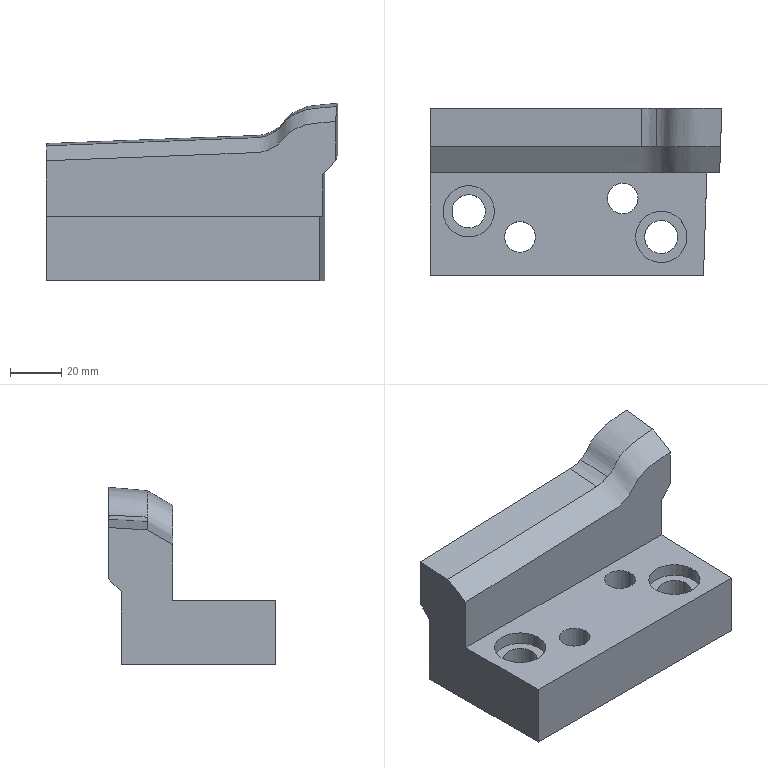Part | NX | features solid 2 | 1 solid | 24 faces | box 113.6 x 65 x 69.113 mm | volume 226886 mm3 | spline 10 | plane 8 | cylinder 6 | commonest cylinder face diameters 12 x2 13 x2 20 x2